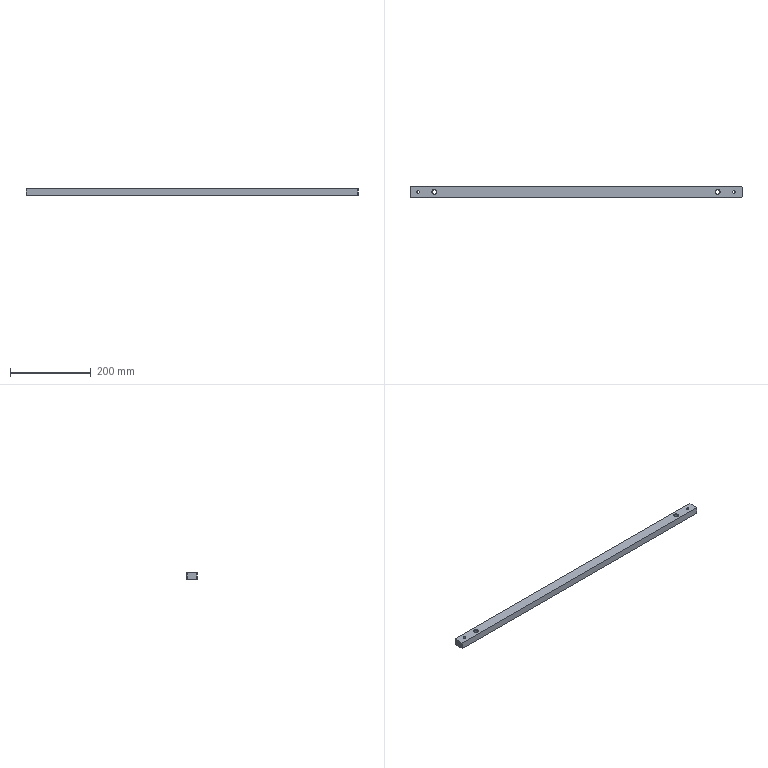Part | NX | features BREP 1 | 1 solid | 48 faces | box 820 x 26 x 17 mm | volume 357246 mm3 | cylinder 20 | cone 16 | plane 12 | commonest cylinder face diameters 3.3 x8 6.6 x4 10 x4 11 x4
STEP:
#1=CARTESIAN_POINT('',(395.5,0.,-1.5));
#2=VERTEX_POINT('',#1);
#3=CARTESIAN_POINT('',(384.5,0.,-1.5));
#4=VERTEX_POINT('',#3);
#5=CARTESIAN_POINT('',(390.,0.,-1.5));
#6=DIRECTION('',(0.,0.,-1.));
#7=DIRECTION('',(-1.,0.,0.));
#8=AXIS2_PLACEMENT_3D('',#5,#6,#7);
#9=CIRCLE('',#8,5.5);
#10=EDGE_CURVE('',#2,#4,#9,.T.);
#11=ORIENTED_EDGE('',*,*,#10,.F.);
#12=CARTESIAN_POINT('',(395.5,0.,-8.5));
#13=VERTEX_POINT('',#12);
#14=CARTESIAN_POINT('',(395.5,0.,-8.5));
#15=DIRECTION('',(0.,0.,-1.));
#16=VECTOR('',#15,1000.);
#17=LINE('',#14,#16);
#18=EDGE_CURVE('',#2,#13,#17,.T.);
#19=ORIENTED_EDGE('',*,*,#18,.T.);
#20=CARTESIAN_POINT('',(384.5,0.,-8.5));
#21=VERTEX_POINT('',#20);
#22=CARTESIAN_POINT('',(390.,0.,-8.5));
#23=DIRECTION('',(0.,0.,-1.));
#24=DIRECTION('',(-1.,0.,0.));
#25=AXIS2_PLACEMENT_3D('',#22,#23,#24);
#26=CIRCLE('',#25,5.5);
#27=EDGE_CURVE('',#13,#21,#26,.T.);
#28=ORIENTED_EDGE('',*,*,#27,.T.);
#29=CARTESIAN_POINT('',(384.5,0.,-8.5));
#30=DIRECTION('',(0.,0.,-1.));
#31=VECTOR('',#30,1000.);
#32=LINE('',#29,#31);
#33=EDGE_CURVE('',#4,#21,#32,.T.);
#34=ORIENTED_EDGE('',*,*,#33,.F.);
#35=EDGE_LOOP('',(#11,#19,#28,#34));
#36=FACE_BOUND('',#35,.T.);
#37=CARTESIAN_POINT('',(390.,0.,-8.5));
#38=DIRECTION('',(0.,0.,-1.));
#39=DIRECTION('',(-1.,0.,0.));
#40=AXIS2_PLACEMENT_3D('',#37,#38,#39);
#41=CYLINDRICAL_SURFACE('',#40,5.5);
#42=ADVANCED_FACE('',(#36),#41,.F.);
#43=CARTESIAN_POINT('',(393.3,0.,8.5));
#44=VERTEX_POINT('',#43);
#45=CARTESIAN_POINT('',(386.7,0.,8.5));
#46=VERTEX_POINT('',#45);
#47=CARTESIAN_POINT('',(390.,0.,8.5));
#48=DIRECTION('',(0.,0.,-1.));
#49=DIRECTION('',(-1.,0.,0.));
#50=AXIS2_PLACEMENT_3D('',#47,#48,#49);
#51=CIRCLE('',#50,3.3);
#52=EDGE_CURVE('',#44,#46,#51,.T.);
#53=ORIENTED_EDGE('',*,*,#52,.F.);
#54=CARTESIAN_POINT('',(393.3,0.,-1.5));
#55=VERTEX_POINT('',#54);
#56=CARTESIAN_POINT('',(393.3,0.,-8.5));
#57=DIRECTION('',(0.,0.,-1.));
#58=VECTOR('',#57,1000.);
#59=LINE('',#56,#58);
#60=EDGE_CURVE('',#44,#55,#59,.T.);
#61=ORIENTED_EDGE('',*,*,#60,.T.);
#62=CARTESIAN_POINT('',(386.7,0.,-1.5));
#63=VERTEX_POINT('',#62);
#64=CARTESIAN_POINT('',(390.,0.,-1.5));
#65=DIRECTION('',(0.,0.,-1.));
#66=DIRECTION('',(-1.,0.,0.));
#67=AXIS2_PLACEMENT_3D('',#64,#65,#66);
#68=CIRCLE('',#67,3.3);
#69=EDGE_CURVE('',#55,#63,#68,.T.);
#70=ORIENTED_EDGE('',*,*,#69,.T.);
#71=CARTESIAN_POINT('',(386.7,0.,-8.5));
#72=DIRECTION('',(0.,0.,-1.));
#73=VECTOR('',#72,1000.);
#74=LINE('',#71,#73);
#75=EDGE_CURVE('',#46,#63,#74,.T.);
#76=ORIENTED_EDGE('',*,*,#75,.F.);
#77=EDGE_LOOP('',(#53,#61,#70,#76));
#78=FACE_BOUND('',#77,.T.);
#79=CARTESIAN_POINT('',(390.,0.,-8.5));
#80=DIRECTION('',(0.,0.,-1.));
#81=DIRECTION('',(-1.,0.,0.));
#82=AXIS2_PLACEMENT_3D('',#79,#80,#81);
#83=CYLINDRICAL_SURFACE('',#82,3.3);
#84=ADVANCED_FACE('',(#78),#83,.F.);
#85=CARTESIAN_POINT('',(-386.7,0.,8.5));
#86=VERTEX_POINT('',#85);
#87=CARTESIAN_POINT('',(-393.3,0.,8.5));
#88=VERTEX_POINT('',#87);
#89=CARTESIAN_POINT('',(-390.,0.,8.5));
#90=DIRECTION('',(0.,0.,-1.));
#91=DIRECTION('',(-1.,0.,0.));
#92=AXIS2_PLACEMENT_3D('',#89,#90,#91);
#93=CIRCLE('',#92,3.3);
#94=EDGE_CURVE('',#86,#88,#93,.T.);
#95=ORIENTED_EDGE('',*,*,#94,.F.);
#96=CARTESIAN_POINT('',(-386.7,0.,-1.5));
#97=VERTEX_POINT('',#96);
#98=CARTESIAN_POINT('',(-386.7,0.,-8.5));
#99=DIRECTION('',(0.,0.,-1.));
#100=VECTOR('',#99,1000.);
#101=LINE('',#98,#100);
#102=EDGE_CURVE('',#86,#97,#101,.T.);
#103=ORIENTED_EDGE('',*,*,#102,.T.);
#104=CARTESIAN_POINT('',(-393.3,0.,-1.5));
#105=VERTEX_POINT('',#104);
#106=CARTESIAN_POINT('',(-390.,0.,-1.5));
#107=DIRECTION('',(0.,0.,-1.));
#108=DIRECTION('',(-1.,0.,0.));
#109=AXIS2_PLACEMENT_3D('',#106,#107,#108);
#110=CIRCLE('',#109,3.3);
#111=EDGE_CURVE('',#97,#105,#110,.T.);
#112=ORIENTED_EDGE('',*,*,#111,.T.);
#113=CARTESIAN_POINT('',(-393.3,0.,-8.5));
#114=DIRECTION('',(0.,0.,-1.));
#115=VECTOR('',#114,1000.);
#116=LINE('',#113,#115);
#117=EDGE_CURVE('',#88,#105,#116,.T.);
#118=ORIENTED_EDGE('',*,*,#117,.F.);
#119=EDGE_LOOP('',(#95,#103,#112,#118));
#120=FACE_BOUND('',#119,.T.);
#121=CARTESIAN_POINT('',(-390.,0.,-8.5));
#122=DIRECTION('',(0.,0.,-1.));
#123=DIRECTION('',(-1.,0.,0.));
#124=AXIS2_PLACEMENT_3D('',#121,#122,#123);
#125=CYLINDRICAL_SURFACE('',#124,3.3);
#126=ADVANCED_FACE('',(#120),#125,.F.);
#127=CARTESIAN_POINT('',(-384.5,0.,-1.5));
#128=VERTEX_POINT('',#127);
#129=CARTESIAN_POINT('',(-395.5,0.,-1.5));
#130=VERTEX_POINT('',#129);
#131=CARTESIAN_POINT('',(-390.,0.,-1.5));
#132=DIRECTION('',(0.,0.,-1.));
#133=DIRECTION('',(-1.,0.,0.));
#134=AXIS2_PLACEMENT_3D('',#131,#132,#133);
#135=CIRCLE('',#134,5.5);
#136=EDGE_CURVE('',#128,#130,#135,.T.);
#137=ORIENTED_EDGE('',*,*,#136,.F.);
#138=CARTESIAN_POINT('',(-384.5,0.,-8.5));
#139=VERTEX_POINT('',#138);
#140=CARTESIAN_POINT('',(-384.5,0.,-8.5));
#141=DIRECTION('',(0.,0.,-1.));
#142=VECTOR('',#141,1000.);
#143=LINE('',#140,#142);
#144=EDGE_CURVE('',#128,#139,#143,.T.);
#145=ORIENTED_EDGE('',*,*,#144,.T.);
#146=CARTESIAN_POINT('',(-395.5,0.,-8.5));
#147=VERTEX_POINT('',#146);
#148=CARTESIAN_POINT('',(-390.,0.,-8.5));
#149=DIRECTION('',(0.,0.,-1.));
#150=DIRECTION('',(-1.,0.,0.));
#151=AXIS2_PLACEMENT_3D('',#148,#149,#150);
#152=CIRCLE('',#151,5.5);
#153=EDGE_CURVE('',#139,#147,#152,.T.);
#154=ORIENTED_EDGE('',*,*,#153,.T.);
#155=CARTESIAN_POINT('',(-395.5,0.,-8.5));
#156=DIRECTION('',(0.,0.,-1.));
#157=VECTOR('',#156,1000.);
#158=LINE('',#155,#157);
#159=EDGE_CURVE('',#130,#147,#158,.T.);
#160=ORIENTED_EDGE('',*,*,#159,.F.);
#161=EDGE_LOOP('',(#137,#145,#154,#160));
#162=FACE_BOUND('',#161,.T.);
#163=CARTESIAN_POINT('',(-390.,0.,-8.5));
#164=DIRECTION('',(0.,0.,-1.));
#165=DIRECTION('',(-1.,0.,0.));
#166=AXIS2_PLACEMENT_3D('',#163,#164,#165);
#167=CYLINDRICAL_SURFACE('',#166,5.5);
#168=ADVANCED_FACE('',(#162),#167,.F.);
#169=CARTESIAN_POINT('',(-355.,0.,7.5));
#170=VERTEX_POINT('',#169);
#171=CARTESIAN_POINT('',(-345.,0.,7.5));
#172=VERTEX_POINT('',#171);
#173=CARTESIAN_POINT('',(-350.,0.,7.5));
#174=DIRECTION('',(0.,0.,1.));
#175=DIRECTION('',(-1.,0.,0.));
#176=AXIS2_PLACEMENT_3D('',#173,#174,#175);
#177=CIRCLE('',#176,5.);
#178=EDGE_CURVE('',#170,#172,#177,.T.);
#179=ORIENTED_EDGE('',*,*,#178,.F.);
#180=CARTESIAN_POINT('',(-356.,0.,8.5));
#181=VERTEX_POINT('',#180);
#182=CARTESIAN_POINT('',(-355.,0.,7.5));
#183=DIRECTION('',(-0.7071,0.,0.7071));
#184=VECTOR('',#183,1000.);
#185=LINE('',#182,#184);
#186=EDGE_CURVE('',#181,#170,#185,.F.);
#187=ORIENTED_EDGE('',*,*,#186,.F.);
#188=CARTESIAN_POINT('',(-344.,0.,8.5));
#189=VERTEX_POINT('',#188);
#190=CARTESIAN_POINT('',(-350.,0.,8.5));
#191=DIRECTION('',(0.,0.,-1.));
#192=DIRECTION('',(-1.,0.,0.));
#193=AXIS2_PLACEMENT_3D('',#190,#191,#192);
#194=CIRCLE('',#193,6.);
#195=EDGE_CURVE('',#189,#181,#194,.T.);
#196=ORIENTED_EDGE('',*,*,#195,.F.);
#197=CARTESIAN_POINT('',(-345.,0.,7.5));
#198=DIRECTION('',(0.7071,0.,0.7071));
#199=VECTOR('',#198,1000.);
#200=LINE('',#197,#199);
#201=EDGE_CURVE('',#189,#172,#200,.F.);
#202=ORIENTED_EDGE('',*,*,#201,.T.);
#203=EDGE_LOOP('',(#179,#187,#196,#202));
#204=FACE_BOUND('',#203,.T.);
#205=CARTESIAN_POINT('',(-350.,0.,7.5));
#206=DIRECTION('',(0.,0.,1.));
#207=DIRECTION('',(1.,0.,0.));
#208=AXIS2_PLACEMENT_3D('',#205,#206,#207);
#209=CONICAL_SURFACE('',#208,5.,0.7854);
#210=ADVANCED_FACE('',(#204),#209,.F.);
#211=CARTESIAN_POINT('',(-345.,0.,-7.5));
#212=VERTEX_POINT('',#211);
#213=CARTESIAN_POINT('',(-355.,0.,-7.5));
#214=VERTEX_POINT('',#213);
#215=CARTESIAN_POINT('',(-350.,0.,-7.5));
#216=DIRECTION('',(0.,0.,-1.));
#217=DIRECTION('',(-1.,0.,0.));
#218=AXIS2_PLACEMENT_3D('',#215,#216,#217);
#219=CIRCLE('',#218,5.);
#220=EDGE_CURVE('',#212,#214,#219,.T.);
#221=ORIENTED_EDGE('',*,*,#220,.F.);
#222=CARTESIAN_POINT('',(-344.,0.,-8.5));
#223=VERTEX_POINT('',#222);
#224=CARTESIAN_POINT('',(-345.,0.,-7.5));
#225=DIRECTION('',(0.7071,0.,-0.7071));
#226=VECTOR('',#225,1000.);
#227=LINE('',#224,#226);
#228=EDGE_CURVE('',#212,#223,#227,.T.);
#229=ORIENTED_EDGE('',*,*,#228,.T.);
#230=CARTESIAN_POINT('',(-356.,0.,-8.5));
#231=VERTEX_POINT('',#230);
#232=CARTESIAN_POINT('',(-350.,0.,-8.5));
#233=DIRECTION('',(0.,0.,1.));
#234=DIRECTION('',(-1.,0.,0.));
#235=AXIS2_PLACEMENT_3D('',#232,#233,#234);
#236=CIRCLE('',#235,6.);
#237=EDGE_CURVE('',#231,#223,#236,.T.);
#238=ORIENTED_EDGE('',*,*,#237,.F.);
#239=CARTESIAN_POINT('',(-355.,0.,-7.5));
#240=DIRECTION('',(-0.7071,0.,-0.7071));
#241=VECTOR('',#240,1000.);
#242=LINE('',#239,#241);
#243=EDGE_CURVE('',#214,#231,#242,.T.);
#244=ORIENTED_EDGE('',*,*,#243,.F.);
#245=EDGE_LOOP('',(#221,#229,#238,#244));
#246=FACE_BOUND('',#245,.T.);
#247=CARTESIAN_POINT('',(-350.,0.,-7.5));
#248=DIRECTION('',(0.,0.,-1.));
#249=DIRECTION('',(-1.,0.,0.));
#250=AXIS2_PLACEMENT_3D('',#247,#248,#249);
#251=CONICAL_SURFACE('',#250,5.,0.7854);
#252=ADVANCED_FACE('',(#246),#251,.F.);
#253=CARTESIAN_POINT('',(345.,0.,7.5));
#254=VERTEX_POINT('',#253);
#255=CARTESIAN_POINT('',(355.,0.,7.5));
#256=VERTEX_POINT('',#255);
#257=CARTESIAN_POINT('',(350.,0.,7.5));
#258=DIRECTION('',(0.,0.,1.));
#259=DIRECTION('',(-1.,0.,0.));
#260=AXIS2_PLACEMENT_3D('',#257,#258,#259);
#261=CIRCLE('',#260,5.);
#262=EDGE_CURVE('',#254,#256,#261,.T.);
#263=ORIENTED_EDGE('',*,*,#262,.F.);
#264=CARTESIAN_POINT('',(344.,0.,8.5));
#265=VERTEX_POINT('',#264);
#266=CARTESIAN_POINT('',(345.,0.,7.5));
#267=DIRECTION('',(-0.7071,0.,0.7071));
#268=VECTOR('',#267,1000.);
#269=LINE('',#266,#268);
#270=EDGE_CURVE('',#265,#254,#269,.F.);
#271=ORIENTED_EDGE('',*,*,#270,.F.);
#272=CARTESIAN_POINT('',(356.,0.,8.5));
#273=VERTEX_POINT('',#272);
#274=CARTESIAN_POINT('',(350.,0.,8.5));
#275=DIRECTION('',(0.,0.,-1.));
#276=DIRECTION('',(-1.,0.,0.));
#277=AXIS2_PLACEMENT_3D('',#274,#275,#276);
#278=CIRCLE('',#277,6.);
#279=EDGE_CURVE('',#273,#265,#278,.T.);
#280=ORIENTED_EDGE('',*,*,#279,.F.);
#281=CARTESIAN_POINT('',(355.,0.,7.5));
#282=DIRECTION('',(0.7071,0.,0.7071));
#283=VECTOR('',#282,1000.);
#284=LINE('',#281,#283);
#285=EDGE_CURVE('',#273,#256,#284,.F.);
#286=ORIENTED_EDGE('',*,*,#285,.T.);
#287=EDGE_LOOP('',(#263,#271,#280,#286));
#288=FACE_BOUND('',#287,.T.);
#289=CARTESIAN_POINT('',(350.,0.,7.5));
#290=DIRECTION('',(0.,0.,1.));
#291=DIRECTION('',(1.,0.,0.));
#292=AXIS2_PLACEMENT_3D('',#289,#290,#291);
#293=CONICAL_SURFACE('',#292,5.,0.7854);
#294=ADVANCED_FACE('',(#288),#293,.F.);
#295=CARTESIAN_POINT('',(355.,0.,-7.5));
#296=VERTEX_POINT('',#295);
#297=CARTESIAN_POINT('',(345.,0.,-7.5));
#298=VERTEX_POINT('',#297);
#299=CARTESIAN_POINT('',(350.,0.,-7.5));
#300=DIRECTION('',(0.,0.,-1.));
#301=DIRECTION('',(-1.,0.,0.));
#302=AXIS2_PLACEMENT_3D('',#299,#300,#301);
#303=CIRCLE('',#302,5.);
#304=EDGE_CURVE('',#296,#298,#303,.T.);
#305=ORIENTED_EDGE('',*,*,#304,.F.);
#306=CARTESIAN_POINT('',(356.,0.,-8.5));
#307=VERTEX_POINT('',#306);
#308=CARTESIAN_POINT('',(355.,0.,-7.5));
#309=DIRECTION('',(0.7071,0.,-0.7071));
#310=VECTOR('',#309,1000.);
#311=LINE('',#308,#310);
#312=EDGE_CURVE('',#296,#307,#311,.T.);
#313=ORIENTED_EDGE('',*,*,#312,.T.);
#314=CARTESIAN_POINT('',(344.,0.,-8.5));
#315=VERTEX_POINT('',#314);
#316=CARTESIAN_POINT('',(350.,0.,-8.5));
#317=DIRECTION('',(0.,0.,1.));
#318=DIRECTION('',(-1.,0.,0.));
#319=AXIS2_PLACEMENT_3D('',#316,#317,#318);
#320=CIRCLE('',#319,6.);
#321=EDGE_CURVE('',#315,#307,#320,.T.);
#322=ORIENTED_EDGE('',*,*,#321,.F.);
#323=CARTESIAN_POINT('',(345.,0.,-7.5));
#324=DIRECTION('',(-0.7071,0.,-0.7071));
#325=VECTOR('',#324,1000.);
#326=LINE('',#323,#325);
#327=EDGE_CURVE('',#298,#315,#326,.T.);
#328=ORIENTED_EDGE('',*,*,#327,.F.);
#329=EDGE_LOOP('',(#305,#313,#322,#328));
#330=FACE_BOUND('',#329,.T.);
#331=CARTESIAN_POINT('',(350.,0.,-7.5));
#332=DIRECTION('',(0.,0.,-1.));
#333=DIRECTION('',(-1.,0.,0.));
#334=AXIS2_PLACEMENT_3D('',#331,#332,#333);
#335=CONICAL_SURFACE('',#334,5.,0.7854);
#336=ADVANCED_FACE('',(#330),#335,.F.);
#337=ORIENTED_EDGE('',*,*,#304,.T.);
#338=CARTESIAN_POINT('',(345.,0.,-174.5));
#339=DIRECTION('',(0.,0.,1.));
#340=VECTOR('',#339,1000.);
#341=LINE('',#338,#340);
#342=EDGE_CURVE('',#254,#298,#341,.F.);
#343=ORIENTED_EDGE('',*,*,#342,.F.);
#344=ORIENTED_EDGE('',*,*,#262,.T.);
#345=CARTESIAN_POINT('',(355.,0.,-174.5));
#346=DIRECTION('',(0.,0.,1.));
#347=VECTOR('',#346,1000.);
#348=LINE('',#345,#347);
#349=EDGE_CURVE('',#256,#296,#348,.F.);
#350=ORIENTED_EDGE('',*,*,#349,.T.);
#351=EDGE_LOOP('',(#337,#343,#344,#350));
#352=FACE_BOUND('',#351,.T.);
#353=CARTESIAN_POINT('',(350.,0.,-174.5));
#354=DIRECTION('',(0.,0.,1.));
#355=DIRECTION('',(1.,0.,0.));
#356=AXIS2_PLACEMENT_3D('',#353,#354,#355);
#357=CYLINDRICAL_SURFACE('',#356,5.);
#358=ADVANCED_FACE('',(#352),#357,.F.);
#359=ORIENTED_EDGE('',*,*,#220,.T.);
#360=CARTESIAN_POINT('',(-355.,0.,-174.5));
#361=DIRECTION('',(0.,0.,1.));
#362=VECTOR('',#361,1000.);
#363=LINE('',#360,#362);
#364=EDGE_CURVE('',#170,#214,#363,.F.);
#365=ORIENTED_EDGE('',*,*,#364,.F.);
#366=ORIENTED_EDGE('',*,*,#178,.T.);
#367=CARTESIAN_POINT('',(-345.,0.,-174.5));
#368=DIRECTION('',(0.,0.,1.));
#369=VECTOR('',#368,1000.);
#370=LINE('',#367,#369);
#371=EDGE_CURVE('',#172,#212,#370,.F.);
#372=ORIENTED_EDGE('',*,*,#371,.T.);
#373=EDGE_LOOP('',(#359,#365,#366,#372));
#374=FACE_BOUND('',#373,.T.);
#375=CARTESIAN_POINT('',(-350.,0.,-174.5));
#376=DIRECTION('',(0.,0.,1.));
#377=DIRECTION('',(1.,0.,0.));
#378=AXIS2_PLACEMENT_3D('',#375,#376,#377);
#379=CYLINDRICAL_SURFACE('',#378,5.);
#380=ADVANCED_FACE('',(#374),#379,.F.);
#381=CARTESIAN_POINT('',(-395.292,1.5,-1.624));
#382=VERTEX_POINT('',#381);
#383=CARTESIAN_POINT('',(-395.,2.291,-1.65));
#384=VERTEX_POINT('',#383);
#385=CARTESIAN_POINT('',(-395.292,1.5,-1.624));
#386=CARTESIAN_POINT('',(-395.214,1.772,-1.638));
#387=CARTESIAN_POINT('',(-395.117,2.036,-1.65));
#388=CARTESIAN_POINT('',(-395.,2.291,-1.65));
#389=B_SPLINE_CURVE_WITH_KNOTS('',3,(#385,#386,#387,#388),.UNSPECIFIED.,.F.,.F.,(4,4),(0.,1.),.UNSPECIFIED.);
#390=EDGE_CURVE('',#382,#384,#389,.T.);
#391=ORIENTED_EDGE('',*,*,#390,.T.);
#392=CARTESIAN_POINT('',(-395.,13.,-1.65));
#393=VERTEX_POINT('',#392);
#394=CARTESIAN_POINT('',(-395.,13.,-1.65));
#395=DIRECTION('',(0.,1.,0.));
#396=VECTOR('',#395,1000.);
#397=LINE('',#394,#396);
#398=EDGE_CURVE('',#384,#393,#397,.T.);
#399=ORIENTED_EDGE('',*,*,#398,.T.);
#400=CARTESIAN_POINT('',(-395.,13.,1.65));
#401=VERTEX_POINT('',#400);
#402=CARTESIAN_POINT('',(-395.,13.,0.));
#403=DIRECTION('',(0.,1.,0.));
#404=DIRECTION('',(0.,0.,1.));
#405=AXIS2_PLACEMENT_3D('',#402,#403,#404);
#406=CIRCLE('',#405,1.65);
#407=EDGE_CURVE('',#393,#401,#406,.T.);
#408=ORIENTED_EDGE('',*,*,#407,.T.);
#409=CARTESIAN_POINT('',(-395.,1.5,1.65));
#410=VERTEX_POINT('',#409);
#411=CARTESIAN_POINT('',(-395.,13.,1.65));
#412=DIRECTION('',(0.,1.,0.));
#413=VECTOR('',#412,1000.);
#414=LINE('',#411,#413);
#415=EDGE_CURVE('',#410,#401,#414,.T.);
#416=ORIENTED_EDGE('',*,*,#415,.F.);
#417=CARTESIAN_POINT('',(-395.,1.5,0.));
#418=DIRECTION('',(0.,1.,0.));
#419=DIRECTION('',(0.,0.,1.));
#420=AXIS2_PLACEMENT_3D('',#417,#418,#419);
#421=CIRCLE('',#420,1.65);
#422=EDGE_CURVE('',#382,#410,#421,.T.);
#423=ORIENTED_EDGE('',*,*,#422,.F.);
#424=EDGE_LOOP('',(#391,#399,#408,#416,#423));
#425=FACE_BOUND('',#424,.T.);
#426=CARTESIAN_POINT('',(-395.,13.,0.));
#427=DIRECTION('',(0.,1.,0.));
#428=DIRECTION('',(0.,0.,1.));
#429=AXIS2_PLACEMENT_3D('',#426,#427,#428);
#430=CYLINDRICAL_SURFACE('',#429,1.65);
#431=ADVANCED_FACE('',(#425),#430,.F.);
#432=CARTESIAN_POINT('',(-395.,0.5086,0.));
#433=VERTEX_POINT('',#432);
#434=CARTESIAN_POINT('',(-395.,1.5,1.65));
#435=DIRECTION('',(0.,0.515,0.8572));
#436=VECTOR('',#435,1000.);
#437=LINE('',#434,#436);
#438=EDGE_CURVE('',#410,#433,#437,.F.);
#439=ORIENTED_EDGE('',*,*,#438,.T.);
#440=CARTESIAN_POINT('',(-395.,1.41,-1.5));
#441=VERTEX_POINT('',#440);
#442=CARTESIAN_POINT('',(-395.,1.5,-1.65));
#443=DIRECTION('',(0.,0.515,-0.8572));
#444=VECTOR('',#443,1000.);
#445=LINE('',#442,#444);
#446=EDGE_CURVE('',#441,#433,#445,.F.);
#447=ORIENTED_EDGE('',*,*,#446,.F.);
#448=CARTESIAN_POINT('',(-395.311,1.429,-1.5));
#449=VERTEX_POINT('',#448);
#450=CARTESIAN_POINT('',(-395.311,1.429,-1.5));
#451=CARTESIAN_POINT('',(-395.206,1.416,-1.5));
#452=CARTESIAN_POINT('',(-395.103,1.41,-1.5));
#453=CARTESIAN_POINT('',(-395.,1.41,-1.5));
#454=B_SPLINE_CURVE_WITH_KNOTS('',3,(#450,#451,#452,#453),.UNSPECIFIED.,.F.,.F.,(4,4),(0.,1.),.UNSPECIFIED.);
#455=EDGE_CURVE('',#441,#449,#454,.F.);
#456=ORIENTED_EDGE('',*,*,#455,.T.);
#457=CARTESIAN_POINT('',(-395.311,1.429,-1.5));
#458=CARTESIAN_POINT('',(-395.305,1.453,-1.541));
#459=CARTESIAN_POINT('',(-395.298,1.476,-1.583));
#460=CARTESIAN_POINT('',(-395.292,1.5,-1.624));
#461=B_SPLINE_CURVE_WITH_KNOTS('',3,(#457,#458,#459,#460),.UNSPECIFIED.,.F.,.F.,(4,4),(0.00001764,0.0001619),.UNSPECIFIED.);
#462=EDGE_CURVE('',#449,#382,#461,.T.);
#463=ORIENTED_EDGE('',*,*,#462,.T.);
#464=ORIENTED_EDGE('',*,*,#422,.T.);
#465=EDGE_LOOP('',(#439,#447,#456,#463,#464));
#466=FACE_BOUND('',#465,.T.);
#467=CARTESIAN_POINT('',(-395.,1.5,0.));
#468=DIRECTION('',(0.,1.,0.));
#469=DIRECTION('',(0.,0.,1.));
#470=AXIS2_PLACEMENT_3D('',#467,#468,#469);
#471=CONICAL_SURFACE('',#470,1.65,1.03);
#472=ADVANCED_FACE('',(#466),#471,.F.);
#473=CARTESIAN_POINT('',(-131.,1.5,-1.65));
#474=VERTEX_POINT('',#473);
#475=CARTESIAN_POINT('',(-131.,1.5,1.65));
#476=VERTEX_POINT('',#475);
#477=CARTESIAN_POINT('',(-131.,1.5,0.));
#478=DIRECTION('',(0.,1.,0.));
#479=DIRECTION('',(0.,0.,1.));
#480=AXIS2_PLACEMENT_3D('',#477,#478,#479);
#481=CIRCLE('',#480,1.65);
#482=EDGE_CURVE('',#474,#476,#481,.T.);
#483=ORIENTED_EDGE('',*,*,#482,.F.);
#484=CARTESIAN_POINT('',(-131.,13.,-1.65));
#485=VERTEX_POINT('',#484);
#486=CARTESIAN_POINT('',(-131.,13.,-1.65));
#487=DIRECTION('',(0.,1.,0.));
#488=VECTOR('',#487,1000.);
#489=LINE('',#486,#488);
#490=EDGE_CURVE('',#485,#474,#489,.F.);
#491=ORIENTED_EDGE('',*,*,#490,.F.);
#492=CARTESIAN_POINT('',(-131.,13.,1.65));
#493=VERTEX_POINT('',#492);
#494=CARTESIAN_POINT('',(-131.,13.,0.));
#495=DIRECTION('',(0.,1.,0.));
#496=DIRECTION('',(0.,0.,1.));
#497=AXIS2_PLACEMENT_3D('',#494,#495,#496);
#498=CIRCLE('',#497,1.65);
#499=EDGE_CURVE('',#485,#493,#498,.T.);
#500=ORIENTED_EDGE('',*,*,#499,.T.);
#501=CARTESIAN_POINT('',(-131.,13.,1.65));
#502=DIRECTION('',(0.,1.,0.));
#503=VECTOR('',#502,1000.);
#504=LINE('',#501,#503);
#505=EDGE_CURVE('',#493,#476,#504,.F.);
#506=ORIENTED_EDGE('',*,*,#505,.T.);
#507=EDGE_LOOP('',(#483,#491,#500,#506));
#508=FACE_BOUND('',#507,.T.);
#509=CARTESIAN_POINT('',(-131.,13.,0.));
#510=DIRECTION('',(0.,1.,0.));
#511=DIRECTION('',(0.,0.,1.));
#512=AXIS2_PLACEMENT_3D('',#509,#510,#511);
#513=CYLINDRICAL_SURFACE('',#512,1.65);
#514=ADVANCED_FACE('',(#508),#513,.F.);
#515=CARTESIAN_POINT('',(-131.,0.5086,0.));
#516=VERTEX_POINT('',#515);
#517=CARTESIAN_POINT('',(-131.,1.5,1.65));
#518=DIRECTION('',(0.,0.515,0.8572));
#519=VECTOR('',#518,1000.);
#520=LINE('',#517,#519);
#521=EDGE_CURVE('',#476,#516,#520,.F.);
#522=ORIENTED_EDGE('',*,*,#521,.T.);
#523=CARTESIAN_POINT('',(-131.,1.5,-1.65));
#524=DIRECTION('',(0.,0.515,-0.8572));
#525=VECTOR('',#524,1000.);
#526=LINE('',#523,#525);
#527=EDGE_CURVE('',#474,#516,#526,.F.);
#528=ORIENTED_EDGE('',*,*,#527,.F.);
#529=ORIENTED_EDGE('',*,*,#482,.T.);
#530=EDGE_LOOP('',(#522,#528,#529));
#531=FACE_BOUND('',#530,.T.);
#532=CARTESIAN_POINT('',(-131.,1.5,0.));
#533=DIRECTION('',(0.,1.,0.));
#534=DIRECTION('',(0.,0.,1.));
#535=AXIS2_PLACEMENT_3D('',#532,#533,#534);
#536=CONICAL_SURFACE('',#535,1.65,1.03);
#537=ADVANCED_FACE('',(#531),#536,.F.);
#538=CARTESIAN_POINT('',(133.,1.5,-1.65));
#539=VERTEX_POINT('',#538);
#540=CARTESIAN_POINT('',(133.,1.5,1.65));
#541=VERTEX_POINT('',#540);
#542=CARTESIAN_POINT('',(133.,1.5,0.));
#543=DIRECTION('',(0.,1.,0.));
#544=DIRECTION('',(0.,0.,1.));
#545=AXIS2_PLACEMENT_3D('',#542,#543,#544);
#546=CIRCLE('',#545,1.65);
#547=EDGE_CURVE('',#539,#541,#546,.T.);
#548=ORIENTED_EDGE('',*,*,#547,.F.);
#549=CARTESIAN_POINT('',(133.,13.,-1.65));
#550=VERTEX_POINT('',#549);
#551=CARTESIAN_POINT('',(133.,13.,-1.65));
#552=DIRECTION('',(0.,1.,0.));
#553=VECTOR('',#552,1000.);
#554=LINE('',#551,#553);
#555=EDGE_CURVE('',#550,#539,#554,.F.);
#556=ORIENTED_EDGE('',*,*,#555,.F.);
#557=CARTESIAN_POINT('',(133.,13.,1.65));
#558=VERTEX_POINT('',#557);
#559=CARTESIAN_POINT('',(133.,13.,0.));
#560=DIRECTION('',(0.,1.,0.));
#561=DIRECTION('',(0.,0.,1.));
#562=AXIS2_PLACEMENT_3D('',#559,#560,#561);
#563=CIRCLE('',#562,1.65);
#564=EDGE_CURVE('',#550,#558,#563,.T.);
#565=ORIENTED_EDGE('',*,*,#564,.T.);
#566=CARTESIAN_POINT('',(133.,13.,1.65));
#567=DIRECTION('',(0.,1.,0.));
#568=VECTOR('',#567,1000.);
#569=LINE('',#566,#568);
#570=EDGE_CURVE('',#558,#541,#569,.F.);
#571=ORIENTED_EDGE('',*,*,#570,.T.);
#572=EDGE_LOOP('',(#548,#556,#565,#571));
#573=FACE_BOUND('',#572,.T.);
#574=CARTESIAN_POINT('',(133.,13.,0.));
#575=DIRECTION('',(0.,1.,0.));
#576=DIRECTION('',(0.,0.,1.));
#577=AXIS2_PLACEMENT_3D('',#574,#575,#576);
#578=CYLINDRICAL_SURFACE('',#577,1.65);
#579=ADVANCED_FACE('',(#573),#578,.F.);
#580=CARTESIAN_POINT('',(133.,0.5086,0.));
#581=VERTEX_POINT('',#580);
#582=CARTESIAN_POINT('',(133.,1.5,1.65));
#583=DIRECTION('',(0.,0.515,0.8572));
#584=VECTOR('',#583,1000.);
#585=LINE('',#582,#584);
#586=EDGE_CURVE('',#541,#581,#585,.F.);
#587=ORIENTED_EDGE('',*,*,#586,.T.);
#588=CARTESIAN_POINT('',(133.,1.5,-1.65));
#589=DIRECTION('',(0.,0.515,-0.8572));
#590=VECTOR('',#589,1000.);
#591=LINE('',#588,#590);
#592=EDGE_CURVE('',#539,#581,#591,.F.);
#593=ORIENTED_EDGE('',*,*,#592,.F.);
#594=ORIENTED_EDGE('',*,*,#547,.T.);
#595=EDGE_LOOP('',(#587,#593,#594));
#596=FACE_BOUND('',#595,.T.);
#597=CARTESIAN_POINT('',(133.,1.5,0.));
#598=DIRECTION('',(0.,1.,0.));
#599=DIRECTION('',(0.,0.,1.));
#600=AXIS2_PLACEMENT_3D('',#597,#598,#599);
#601=CONICAL_SURFACE('',#600,1.65,1.03);
#602=ADVANCED_FACE('',(#596),#601,.F.);
#603=CARTESIAN_POINT('',(397.,1.5,-1.65));
#604=VERTEX_POINT('',#603);
#605=CARTESIAN_POINT('',(397.,1.5,1.65));
#606=VERTEX_POINT('',#605);
#607=CARTESIAN_POINT('',(397.,1.5,0.));
#608=DIRECTION('',(0.,1.,0.));
#609=DIRECTION('',(0.,0.,1.));
#610=AXIS2_PLACEMENT_3D('',#607,#608,#609);
#611=CIRCLE('',#610,1.65);
#612=EDGE_CURVE('',#604,#606,#611,.T.);
#613=ORIENTED_EDGE('',*,*,#612,.F.);
#614=CARTESIAN_POINT('',(397.,13.,-1.65));
#615=VERTEX_POINT('',#614);
#616=CARTESIAN_POINT('',(397.,13.,-1.65));
#617=DIRECTION('',(0.,1.,0.));
#618=VECTOR('',#617,1000.);
#619=LINE('',#616,#618);
#620=EDGE_CURVE('',#615,#604,#619,.F.);
#621=ORIENTED_EDGE('',*,*,#620,.F.);
#622=CARTESIAN_POINT('',(397.,13.,1.65));
#623=VERTEX_POINT('',#622);
#624=CARTESIAN_POINT('',(397.,13.,0.));
#625=DIRECTION('',(0.,1.,0.));
#626=DIRECTION('',(0.,0.,1.));
#627=AXIS2_PLACEMENT_3D('',#624,#625,#626);
#628=CIRCLE('',#627,1.65);
#629=EDGE_CURVE('',#615,#623,#628,.T.);
#630=ORIENTED_EDGE('',*,*,#629,.T.);
#631=CARTESIAN_POINT('',(397.,13.,1.65));
#632=DIRECTION('',(0.,1.,0.));
#633=VECTOR('',#632,1000.);
#634=LINE('',#631,#633);
#635=EDGE_CURVE('',#623,#606,#634,.F.);
#636=ORIENTED_EDGE('',*,*,#635,.T.);
#637=EDGE_LOOP('',(#613,#621,#630,#636));
#638=FACE_BOUND('',#637,.T.);
#639=CARTESIAN_POINT('',(397.,13.,0.));
#640=DIRECTION('',(0.,1.,0.));
#641=DIRECTION('',(0.,0.,1.));
#642=AXIS2_PLACEMENT_3D('',#639,#640,#641);
#643=CYLINDRICAL_SURFACE('',#642,1.65);
#644=ADVANCED_FACE('',(#638),#643,.F.);
#645=CARTESIAN_POINT('',(397.,0.5086,0.));
#646=VERTEX_POINT('',#645);
#647=CARTESIAN_POINT('',(397.,1.5,1.65));
#648=DIRECTION('',(0.,0.515,0.8572));
#649=VECTOR('',#648,1000.);
#650=LINE('',#647,#649);
#651=EDGE_CURVE('',#606,#646,#650,.F.);
#652=ORIENTED_EDGE('',*,*,#651,.T.);
#653=CARTESIAN_POINT('',(397.,1.5,-1.65));
#654=DIRECTION('',(0.,0.515,-0.8572));
#655=VECTOR('',#654,1000.);
#656=LINE('',#653,#655);
#657=EDGE_CURVE('',#604,#646,#656,.F.);
#658=ORIENTED_EDGE('',*,*,#657,.F.);
#659=ORIENTED_EDGE('',*,*,#612,.T.);
#660=EDGE_LOOP('',(#652,#658,#659));
#661=FACE_BOUND('',#660,.T.);
#662=CARTESIAN_POINT('',(397.,1.5,0.));
#663=DIRECTION('',(0.,1.,0.));
#664=DIRECTION('',(0.,0.,1.));
#665=AXIS2_PLACEMENT_3D('',#662,#663,#664);
#666=CONICAL_SURFACE('',#665,1.65,1.03);
#667=ADVANCED_FACE('',(#661),#666,.F.);
#668=CARTESIAN_POINT('',(410.,-12.,8.5));
#669=VERTEX_POINT('',#668);
#670=CARTESIAN_POINT('',(410.,12.,8.5));
#671=VERTEX_POINT('',#670);
#672=CARTESIAN_POINT('',(410.,-13.,8.5));
#673=DIRECTION('',(0.,1.,0.));
#674=VECTOR('',#673,1000.);
#675=LINE('',#672,#674);
#676=EDGE_CURVE('',#669,#671,#675,.T.);
#677=ORIENTED_EDGE('',*,*,#676,.F.);
#678=CARTESIAN_POINT('',(410.,-12.,-8.5));
#679=VERTEX_POINT('',#678);
#680=CARTESIAN_POINT('',(410.,-12.,8.5));
#681=DIRECTION('',(0.,0.,-1.));
#682=VECTOR('',#681,1000.);
#683=LINE('',#680,#682);
#684=EDGE_CURVE('',#669,#679,#683,.T.);
#685=ORIENTED_EDGE('',*,*,#684,.T.);
#686=CARTESIAN_POINT('',(410.,12.,-8.5));
#687=VERTEX_POINT('',#686);
#688=CARTESIAN_POINT('',(410.,-13.,-8.5));
#689=DIRECTION('',(0.,1.,0.));
#690=VECTOR('',#689,1000.);
#691=LINE('',#688,#690);
#692=EDGE_CURVE('',#679,#687,#691,.T.);
#693=ORIENTED_EDGE('',*,*,#692,.T.);
#694=CARTESIAN_POINT('',(410.,12.,8.5));
#695=DIRECTION('',(0.,0.,1.));
#696=VECTOR('',#695,1000.);
#697=LINE('',#694,#696);
#698=EDGE_CURVE('',#687,#671,#697,.T.);
#699=ORIENTED_EDGE('',*,*,#698,.T.);
#700=EDGE_LOOP('',(#677,#685,#693,#699));
#701=FACE_BOUND('',#700,.T.);
#702=CARTESIAN_POINT('',(410.,-13.,8.5));
#703=DIRECTION('',(-1.,0.,0.));
#704=DIRECTION('',(0.,0.,1.));
#705=AXIS2_PLACEMENT_3D('',#702,#703,#704);
#706=PLANE('',#705);
#707=ADVANCED_FACE('',(#701),#706,.F.);
#708=CARTESIAN_POINT('',(409.,13.,8.5));
#709=VERTEX_POINT('',#708);
#710=CARTESIAN_POINT('',(-409.,13.,8.5));
#711=VERTEX_POINT('',#710);
#712=CARTESIAN_POINT('',(-410.,13.,8.5));
#713=DIRECTION('',(-1.,0.,0.));
#714=VECTOR('',#713,1000.);
#715=LINE('',#712,#714);
#716=EDGE_CURVE('',#709,#711,#715,.T.);
#717=ORIENTED_EDGE('',*,*,#716,.F.);
#718=CARTESIAN_POINT('',(409.,13.,-8.5));
#719=VERTEX_POINT('',#718);
#720=CARTESIAN_POINT('',(409.,13.,8.5));
#721=DIRECTION('',(0.,0.,-1.));
#722=VECTOR('',#721,1000.);
#723=LINE('',#720,#722);
#724=EDGE_CURVE('',#709,#719,#723,.T.);
#725=ORIENTED_EDGE('',*,*,#724,.T.);
#726=CARTESIAN_POINT('',(-409.,13.,-8.5));
#727=VERTEX_POINT('',#726);
#728=CARTESIAN_POINT('',(-410.,13.,-8.5));
#729=DIRECTION('',(-1.,0.,0.));
#730=VECTOR('',#729,1000.);
#731=LINE('',#728,#730);
#732=EDGE_CURVE('',#719,#727,#731,.T.);
#733=ORIENTED_EDGE('',*,*,#732,.T.);
#734=CARTESIAN_POINT('',(-409.,13.,8.5));
#735=DIRECTION('',(0.,0.,1.));
#736=VECTOR('',#735,1000.);
#737=LINE('',#734,#736);
#738=EDGE_CURVE('',#727,#711,#737,.T.);
#739=ORIENTED_EDGE('',*,*,#738,.T.);
#740=EDGE_LOOP('',(#717,#725,#733,#739));
#741=FACE_BOUND('',#740,.T.);
#742=CARTESIAN_POINT('',(-395.,13.,0.));
#743=DIRECTION('',(0.,1.,0.));
#744=DIRECTION('',(0.,0.,1.));
#745=AXIS2_PLACEMENT_3D('',#742,#743,#744);
#746=CIRCLE('',#745,1.65);
#747=EDGE_CURVE('',#401,#393,#746,.T.);
#748=ORIENTED_EDGE('',*,*,#747,.F.);
#749=ORIENTED_EDGE('',*,*,#407,.F.);
#750=EDGE_LOOP('',(#748,#749));
#751=FACE_BOUND('',#750,.T.);
#752=CARTESIAN_POINT('',(-131.,13.,0.));
#753=DIRECTION('',(0.,1.,0.));
#754=DIRECTION('',(0.,0.,1.));
#755=AXIS2_PLACEMENT_3D('',#752,#753,#754);
#756=CIRCLE('',#755,1.65);
#757=EDGE_CURVE('',#493,#485,#756,.T.);
#758=ORIENTED_EDGE('',*,*,#757,.F.);
#759=ORIENTED_EDGE('',*,*,#499,.F.);
#760=EDGE_LOOP('',(#758,#759));
#761=FACE_BOUND('',#760,.T.);
#762=CARTESIAN_POINT('',(133.,13.,0.));
#763=DIRECTION('',(0.,1.,0.));
#764=DIRECTION('',(0.,0.,1.));
#765=AXIS2_PLACEMENT_3D('',#762,#763,#764);
#766=CIRCLE('',#765,1.65);
#767=EDGE_CURVE('',#558,#550,#766,.T.);
#768=ORIENTED_EDGE('',*,*,#767,.F.);
#769=ORIENTED_EDGE('',*,*,#564,.F.);
#770=EDGE_LOOP('',(#768,#769));
#771=FACE_BOUND('',#770,.T.);
#772=CARTESIAN_POINT('',(397.,13.,0.));
#773=DIRECTION('',(0.,1.,0.));
#774=DIRECTION('',(0.,0.,1.));
#775=AXIS2_PLACEMENT_3D('',#772,#773,#774);
#776=CIRCLE('',#775,1.65);
#777=EDGE_CURVE('',#623,#615,#776,.T.);
#778=ORIENTED_EDGE('',*,*,#777,.F.);
#779=ORIENTED_EDGE('',*,*,#629,.F.);
#780=EDGE_LOOP('',(#778,#779));
#781=FACE_BOUND('',#780,.T.);
#782=CARTESIAN_POINT('',(-410.,13.,8.5));
#783=DIRECTION('',(0.,-1.,0.));
#784=DIRECTION('',(0.,0.,-1.));
#785=AXIS2_PLACEMENT_3D('',#782,#783,#784);
#786=PLANE('',#785);
#787=ADVANCED_FACE('',(#741,#751,#761,#771,#781),#786,.F.);
#788=CARTESIAN_POINT('',(-410.,12.,-8.5));
#789=VERTEX_POINT('',#788);
#790=CARTESIAN_POINT('',(-410.,-12.,-8.5));
#791=VERTEX_POINT('',#790);
#792=CARTESIAN_POINT('',(-410.,-13.,-8.5));
#793=DIRECTION('',(0.,-1.,0.));
#794=VECTOR('',#793,1000.);
#795=LINE('',#792,#794);
#796=EDGE_CURVE('',#789,#791,#795,.T.);
#797=ORIENTED_EDGE('',*,*,#796,.T.);
#798=CARTESIAN_POINT('',(-410.,-12.,8.5));
#799=VERTEX_POINT('',#798);
#800=CARTESIAN_POINT('',(-410.,-12.,8.5));
#801=DIRECTION('',(0.,0.,1.));
#802=VECTOR('',#801,1000.);
#803=LINE('',#800,#802);
#804=EDGE_CURVE('',#791,#799,#803,.T.);
#805=ORIENTED_EDGE('',*,*,#804,.T.);
#806=CARTESIAN_POINT('',(-410.,12.,8.5));
#807=VERTEX_POINT('',#806);
#808=CARTESIAN_POINT('',(-410.,-13.,8.5));
#809=DIRECTION('',(0.,-1.,0.));
#810=VECTOR('',#809,1000.);
#811=LINE('',#808,#810);
#812=EDGE_CURVE('',#807,#799,#811,.T.);
#813=ORIENTED_EDGE('',*,*,#812,.F.);
#814=CARTESIAN_POINT('',(-410.,12.,8.5));
#815=DIRECTION('',(0.,0.,-1.));
#816=VECTOR('',#815,1000.);
#817=LINE('',#814,#816);
#818=EDGE_CURVE('',#807,#789,#817,.T.);
#819=ORIENTED_EDGE('',*,*,#818,.T.);
#820=EDGE_LOOP('',(#797,#805,#813,#819));
#821=FACE_BOUND('',#820,.T.);
#822=CARTESIAN_POINT('',(-410.,-13.,8.5));
#823=DIRECTION('',(1.,0.,0.));
#824=DIRECTION('',(0.,1.,0.));
#825=AXIS2_PLACEMENT_3D('',#822,#823,#824);
#826=PLANE('',#825);
#827=ADVANCED_FACE('',(#821),#826,.F.);
#828=CARTESIAN_POINT('',(-409.,-13.,-8.5));
#829=VERTEX_POINT('',#828);
#830=CARTESIAN_POINT('',(409.,-13.,-8.5));
#831=VERTEX_POINT('',#830);
#832=CARTESIAN_POINT('',(-410.,-13.,-8.5));
#833=DIRECTION('',(1.,0.,0.));
#834=VECTOR('',#833,1000.);
#835=LINE('',#832,#834);
#836=EDGE_CURVE('',#829,#831,#835,.T.);
#837=ORIENTED_EDGE('',*,*,#836,.T.);
#838=CARTESIAN_POINT('',(409.,-13.,8.5));
#839=VERTEX_POINT('',#838);
#840=CARTESIAN_POINT('',(409.,-13.,8.5));
#841=DIRECTION('',(0.,0.,1.));
#842=VECTOR('',#841,1000.);
#843=LINE('',#840,#842);
#844=EDGE_CURVE('',#831,#839,#843,.T.);
#845=ORIENTED_EDGE('',*,*,#844,.T.);
#846=CARTESIAN_POINT('',(-409.,-13.,8.5));
#847=VERTEX_POINT('',#846);
#848=CARTESIAN_POINT('',(-410.,-13.,8.5));
#849=DIRECTION('',(1.,0.,0.));
#850=VECTOR('',#849,1000.);
#851=LINE('',#848,#850);
#852=EDGE_CURVE('',#847,#839,#851,.T.);
#853=ORIENTED_EDGE('',*,*,#852,.F.);
#854=CARTESIAN_POINT('',(-409.,-13.,8.5));
#855=DIRECTION('',(0.,0.,-1.));
#856=VECTOR('',#855,1000.);
#857=LINE('',#854,#856);
#858=EDGE_CURVE('',#847,#829,#857,.T.);
#859=ORIENTED_EDGE('',*,*,#858,.T.);
#860=EDGE_LOOP('',(#837,#845,#853,#859));
#861=FACE_BOUND('',#860,.T.);
#862=CARTESIAN_POINT('',(-410.,-13.,8.5));
#863=DIRECTION('',(0.,1.,0.));
#864=DIRECTION('',(1.,0.,0.));
#865=AXIS2_PLACEMENT_3D('',#862,#863,#864);
#866=PLANE('',#865);
#867=ADVANCED_FACE('',(#861),#866,.F.);
#868=ORIENTED_EDGE('',*,*,#852,.T.);
#869=CARTESIAN_POINT('',(410.,-12.,8.5));
#870=DIRECTION('',(0.7071,0.7071,0.));
#871=VECTOR('',#870,1000.);
#872=LINE('',#869,#871);
#873=EDGE_CURVE('',#839,#669,#872,.T.);
#874=ORIENTED_EDGE('',*,*,#873,.T.);
#875=ORIENTED_EDGE('',*,*,#676,.T.);
#876=CARTESIAN_POINT('',(409.,13.,8.5));
#877=DIRECTION('',(-0.7071,0.7071,0.));
#878=VECTOR('',#877,1000.);
#879=LINE('',#876,#878);
#880=EDGE_CURVE('',#671,#709,#879,.T.);
#881=ORIENTED_EDGE('',*,*,#880,.T.);
#882=ORIENTED_EDGE('',*,*,#716,.T.);
#883=CARTESIAN_POINT('',(-410.,12.,8.5));
#884=DIRECTION('',(-0.7071,-0.7071,0.));
#885=VECTOR('',#884,1000.);
#886=LINE('',#883,#885);
#887=EDGE_CURVE('',#711,#807,#886,.T.);
#888=ORIENTED_EDGE('',*,*,#887,.T.);
#889=ORIENTED_EDGE('',*,*,#812,.T.);
#890=CARTESIAN_POINT('',(-409.,-13.,8.5));
#891=DIRECTION('',(0.7071,-0.7071,0.));
#892=VECTOR('',#891,1000.);
#893=LINE('',#890,#892);
#894=EDGE_CURVE('',#799,#847,#893,.T.);
#895=ORIENTED_EDGE('',*,*,#894,.T.);
#896=EDGE_LOOP('',(#868,#874,#875,#881,#882,#888,#889,#895));
#897=FACE_BOUND('',#896,.T.);
#898=CARTESIAN_POINT('',(390.,0.,8.5));
#899=DIRECTION('',(0.,0.,-1.));
#900=DIRECTION('',(-1.,0.,0.));
#901=AXIS2_PLACEMENT_3D('',#898,#899,#900);
#902=CIRCLE('',#901,3.3);
#903=EDGE_CURVE('',#46,#44,#902,.T.);
#904=ORIENTED_EDGE('',*,*,#903,.T.);
#905=ORIENTED_EDGE('',*,*,#52,.T.);
#906=EDGE_LOOP('',(#904,#905));
#907=FACE_BOUND('',#906,.T.);
#908=CARTESIAN_POINT('',(-390.,0.,8.5));
#909=DIRECTION('',(0.,0.,-1.));
#910=DIRECTION('',(-1.,0.,0.));
#911=AXIS2_PLACEMENT_3D('',#908,#909,#910);
#912=CIRCLE('',#911,3.3);
#913=EDGE_CURVE('',#88,#86,#912,.T.);
#914=ORIENTED_EDGE('',*,*,#913,.T.);
#915=ORIENTED_EDGE('',*,*,#94,.T.);
#916=EDGE_LOOP('',(#914,#915));
#917=FACE_BOUND('',#916,.T.);
#918=ORIENTED_EDGE('',*,*,#279,.T.);
#919=CARTESIAN_POINT('',(350.,0.,8.5));
#920=DIRECTION('',(0.,0.,-1.));
#921=DIRECTION('',(-1.,0.,0.));
#922=AXIS2_PLACEMENT_3D('',#919,#920,#921);
#923=CIRCLE('',#922,6.);
#924=EDGE_CURVE('',#265,#273,#923,.T.);
#925=ORIENTED_EDGE('',*,*,#924,.T.);
#926=EDGE_LOOP('',(#918,#925));
#927=FACE_BOUND('',#926,.T.);
#928=ORIENTED_EDGE('',*,*,#195,.T.);
#929=CARTESIAN_POINT('',(-350.,0.,8.5));
#930=DIRECTION('',(0.,0.,-1.));
#931=DIRECTION('',(-1.,0.,0.));
#932=AXIS2_PLACEMENT_3D('',#929,#930,#931);
#933=CIRCLE('',#932,6.);
#934=EDGE_CURVE('',#181,#189,#933,.T.);
#935=ORIENTED_EDGE('',*,*,#934,.T.);
#936=EDGE_LOOP('',(#928,#935));
#937=FACE_BOUND('',#936,.T.);
#938=CARTESIAN_POINT('',(0.,0.,8.5));
#939=DIRECTION('',(0.,0.,-1.));
#940=DIRECTION('',(0.,-1.,0.));
#941=AXIS2_PLACEMENT_3D('',#938,#939,#940);
#942=PLANE('',#941);
#943=ADVANCED_FACE('',(#897,#907,#917,#927,#937),#942,.F.);
#944=ORIENTED_EDGE('',*,*,#692,.F.);
#945=CARTESIAN_POINT('',(211.,-211.,-8.5));
#946=DIRECTION('',(-0.7071,-0.7071,0.));
#947=VECTOR('',#946,1000.);
#948=LINE('',#945,#947);
#949=EDGE_CURVE('',#679,#831,#948,.T.);
#950=ORIENTED_EDGE('',*,*,#949,.T.);
#951=ORIENTED_EDGE('',*,*,#836,.F.);
#952=CARTESIAN_POINT('',(-211.,-211.,-8.5));
#953=DIRECTION('',(-0.7071,0.7071,0.));
#954=VECTOR('',#953,1000.);
#955=LINE('',#952,#954);
#956=EDGE_CURVE('',#829,#791,#955,.T.);
#957=ORIENTED_EDGE('',*,*,#956,.T.);
#958=ORIENTED_EDGE('',*,*,#796,.F.);
#959=CARTESIAN_POINT('',(-211.,211.,-8.5));
#960=DIRECTION('',(0.7071,0.7071,0.));
#961=VECTOR('',#960,1000.);
#962=LINE('',#959,#961);
#963=EDGE_CURVE('',#789,#727,#962,.T.);
#964=ORIENTED_EDGE('',*,*,#963,.T.);
#965=ORIENTED_EDGE('',*,*,#732,.F.);
#966=CARTESIAN_POINT('',(211.,211.,-8.5));
#967=DIRECTION('',(0.7071,-0.7071,0.));
#968=VECTOR('',#967,1000.);
#969=LINE('',#966,#968);
#970=EDGE_CURVE('',#719,#687,#969,.T.);
#971=ORIENTED_EDGE('',*,*,#970,.T.);
#972=EDGE_LOOP('',(#944,#950,#951,#957,#958,#964,#965,#971));
#973=FACE_BOUND('',#972,.T.);
#974=CARTESIAN_POINT('',(390.,0.,-8.5));
#975=DIRECTION('',(0.,0.,-1.));
#976=DIRECTION('',(-1.,0.,0.));
#977=AXIS2_PLACEMENT_3D('',#974,#975,#976);
#978=CIRCLE('',#977,5.5);
#979=EDGE_CURVE('',#21,#13,#978,.T.);
#980=ORIENTED_EDGE('',*,*,#979,.F.);
#981=ORIENTED_EDGE('',*,*,#27,.F.);
#982=EDGE_LOOP('',(#980,#981));
#983=FACE_BOUND('',#982,.T.);
#984=CARTESIAN_POINT('',(-390.,0.,-8.5));
#985=DIRECTION('',(0.,0.,-1.));
#986=DIRECTION('',(-1.,0.,0.));
#987=AXIS2_PLACEMENT_3D('',#984,#985,#986);
#988=CIRCLE('',#987,5.5);
#989=EDGE_CURVE('',#147,#139,#988,.T.);
#990=ORIENTED_EDGE('',*,*,#989,.F.);
#991=ORIENTED_EDGE('',*,*,#153,.F.);
#992=EDGE_LOOP('',(#990,#991));
#993=FACE_BOUND('',#992,.T.);
#994=ORIENTED_EDGE('',*,*,#321,.T.);
#995=CARTESIAN_POINT('',(350.,0.,-8.5));
#996=DIRECTION('',(0.,0.,1.));
#997=DIRECTION('',(-1.,0.,0.));
#998=AXIS2_PLACEMENT_3D('',#995,#996,#997);
#999=CIRCLE('',#998,6.);
#1000=EDGE_CURVE('',#307,#315,#999,.T.);
#1001=ORIENTED_EDGE('',*,*,#1000,.T.);
#1002=EDGE_LOOP('',(#994,#1001));
#1003=FACE_BOUND('',#1002,.T.);
#1004=ORIENTED_EDGE('',*,*,#237,.T.);
#1005=CARTESIAN_POINT('',(-350.,0.,-8.5));
#1006=DIRECTION('',(0.,0.,1.));
#1007=DIRECTION('',(-1.,0.,0.));
#1008=AXIS2_PLACEMENT_3D('',#1005,#1006,#1007);
#1009=CIRCLE('',#1008,6.);
#1010=EDGE_CURVE('',#223,#231,#1009,.T.);
#1011=ORIENTED_EDGE('',*,*,#1010,.T.);
#1012=EDGE_LOOP('',(#1004,#1011));
#1013=FACE_BOUND('',#1012,.T.);
#1014=CARTESIAN_POINT('',(0.,0.,-8.5));
#1015=DIRECTION('',(0.,0.,-1.));
#1016=DIRECTION('',(0.,-1.,0.));
#1017=AXIS2_PLACEMENT_3D('',#1014,#1015,#1016);
#1018=PLANE('',#1017);
#1019=ADVANCED_FACE('',(#973,#983,#993,#1003,#1013),#1018,.T.);
#1020=ORIENTED_EDGE('',*,*,#657,.T.);
#1021=ORIENTED_EDGE('',*,*,#651,.F.);
#1022=CARTESIAN_POINT('',(397.,1.5,0.));
#1023=DIRECTION('',(0.,1.,0.));
#1024=DIRECTION('',(0.,0.,1.));
#1025=AXIS2_PLACEMENT_3D('',#1022,#1023,#1024);
#1026=CIRCLE('',#1025,1.65);
#1027=EDGE_CURVE('',#606,#604,#1026,.T.);
#1028=ORIENTED_EDGE('',*,*,#1027,.T.);
#1029=EDGE_LOOP('',(#1020,#1021,#1028));
#1030=FACE_BOUND('',#1029,.T.);
#1031=CARTESIAN_POINT('',(397.,1.5,0.));
#1032=DIRECTION('',(0.,1.,0.));
#1033=DIRECTION('',(0.,0.,1.));
#1034=AXIS2_PLACEMENT_3D('',#1031,#1032,#1033);
#1035=CONICAL_SURFACE('',#1034,1.65,1.03);
#1036=ADVANCED_FACE('',(#1030),#1035,.F.);
#1037=ORIENTED_EDGE('',*,*,#620,.T.);
#1038=ORIENTED_EDGE('',*,*,#1027,.F.);
#1039=ORIENTED_EDGE('',*,*,#635,.F.);
#1040=ORIENTED_EDGE('',*,*,#777,.T.);
#1041=EDGE_LOOP('',(#1037,#1038,#1039,#1040));
#1042=FACE_BOUND('',#1041,.T.);
#1043=CARTESIAN_POINT('',(397.,13.,0.));
#1044=DIRECTION('',(0.,1.,0.));
#1045=DIRECTION('',(0.,0.,1.));
#1046=AXIS2_PLACEMENT_3D('',#1043,#1044,#1045);
#1047=CYLINDRICAL_SURFACE('',#1046,1.65);
#1048=ADVANCED_FACE('',(#1042),#1047,.F.);
#1049=ORIENTED_EDGE('',*,*,#592,.T.);
#1050=ORIENTED_EDGE('',*,*,#586,.F.);
#1051=CARTESIAN_POINT('',(133.,1.5,0.));
#1052=DIRECTION('',(0.,1.,0.));
#1053=DIRECTION('',(0.,0.,1.));
#1054=AXIS2_PLACEMENT_3D('',#1051,#1052,#1053);
#1055=CIRCLE('',#1054,1.65);
#1056=EDGE_CURVE('',#541,#539,#1055,.T.);
#1057=ORIENTED_EDGE('',*,*,#1056,.T.);
#1058=EDGE_LOOP('',(#1049,#1050,#1057));
#1059=FACE_BOUND('',#1058,.T.);
#1060=CARTESIAN_POINT('',(133.,1.5,0.));
#1061=DIRECTION('',(0.,1.,0.));
#1062=DIRECTION('',(0.,0.,1.));
#1063=AXIS2_PLACEMENT_3D('',#1060,#1061,#1062);
#1064=CONICAL_SURFACE('',#1063,1.65,1.03);
#1065=ADVANCED_FACE('',(#1059),#1064,.F.);
#1066=ORIENTED_EDGE('',*,*,#555,.T.);
#1067=ORIENTED_EDGE('',*,*,#1056,.F.);
#1068=ORIENTED_EDGE('',*,*,#570,.F.);
#1069=ORIENTED_EDGE('',*,*,#767,.T.);
#1070=EDGE_LOOP('',(#1066,#1067,#1068,#1069));
#1071=FACE_BOUND('',#1070,.T.);
#1072=CARTESIAN_POINT('',(133.,13.,0.));
#1073=DIRECTION('',(0.,1.,0.));
#1074=DIRECTION('',(0.,0.,1.));
#1075=AXIS2_PLACEMENT_3D('',#1072,#1073,#1074);
#1076=CYLINDRICAL_SURFACE('',#1075,1.65);
#1077=ADVANCED_FACE('',(#1071),#1076,.F.);
#1078=ORIENTED_EDGE('',*,*,#527,.T.);
#1079=ORIENTED_EDGE('',*,*,#521,.F.);
#1080=CARTESIAN_POINT('',(-131.,1.5,0.));
#1081=DIRECTION('',(0.,1.,0.));
#1082=DIRECTION('',(0.,0.,1.));
#1083=AXIS2_PLACEMENT_3D('',#1080,#1081,#1082);
#1084=CIRCLE('',#1083,1.65);
#1085=EDGE_CURVE('',#476,#474,#1084,.T.);
#1086=ORIENTED_EDGE('',*,*,#1085,.T.);
#1087=EDGE_LOOP('',(#1078,#1079,#1086));
#1088=FACE_BOUND('',#1087,.T.);
#1089=CARTESIAN_POINT('',(-131.,1.5,0.));
#1090=DIRECTION('',(0.,1.,0.));
#1091=DIRECTION('',(0.,0.,1.));
#1092=AXIS2_PLACEMENT_3D('',#1089,#1090,#1091);
#1093=CONICAL_SURFACE('',#1092,1.65,1.03);
#1094=ADVANCED_FACE('',(#1088),#1093,.F.);
#1095=ORIENTED_EDGE('',*,*,#490,.T.);
#1096=ORIENTED_EDGE('',*,*,#1085,.F.);
#1097=ORIENTED_EDGE('',*,*,#505,.F.);
#1098=ORIENTED_EDGE('',*,*,#757,.T.);
#1099=EDGE_LOOP('',(#1095,#1096,#1097,#1098));
#1100=FACE_BOUND('',#1099,.T.);
#1101=CARTESIAN_POINT('',(-131.,13.,0.));
#1102=DIRECTION('',(0.,1.,0.));
#1103=DIRECTION('',(0.,0.,1.));
#1104=AXIS2_PLACEMENT_3D('',#1101,#1102,#1103);
#1105=CYLINDRICAL_SURFACE('',#1104,1.65);
#1106=ADVANCED_FACE('',(#1100),#1105,.F.);
#1107=ORIENTED_EDGE('',*,*,#446,.T.);
#1108=ORIENTED_EDGE('',*,*,#438,.F.);
#1109=CARTESIAN_POINT('',(-394.313,1.5,-1.5));
#1110=VERTEX_POINT('',#1109);
#1111=CARTESIAN_POINT('',(-395.,1.5,0.));
#1112=DIRECTION('',(0.,1.,0.));
#1113=DIRECTION('',(0.,0.,1.));
#1114=AXIS2_PLACEMENT_3D('',#1111,#1112,#1113);
#1115=CIRCLE('',#1114,1.65);
#1116=EDGE_CURVE('',#410,#1110,#1115,.T.);
#1117=ORIENTED_EDGE('',*,*,#1116,.T.);
#1118=CARTESIAN_POINT('',(-395.,1.41,-1.5));
#1119=CARTESIAN_POINT('',(-394.782,1.41,-1.5));
#1120=CARTESIAN_POINT('',(-394.553,1.44,-1.5));
#1121=CARTESIAN_POINT('',(-394.313,1.5,-1.5));
#1122=B_SPLINE_CURVE_WITH_KNOTS('',3,(#1118,#1119,#1120,#1121),.UNSPECIFIED.,.F.,.F.,(4,4),(0.,1.),.UNSPECIFIED.);
#1123=EDGE_CURVE('',#1110,#441,#1122,.F.);
#1124=ORIENTED_EDGE('',*,*,#1123,.T.);
#1125=EDGE_LOOP('',(#1107,#1108,#1117,#1124));
#1126=FACE_BOUND('',#1125,.T.);
#1127=CARTESIAN_POINT('',(-395.,1.5,0.));
#1128=DIRECTION('',(0.,1.,0.));
#1129=DIRECTION('',(0.,0.,1.));
#1130=AXIS2_PLACEMENT_3D('',#1127,#1128,#1129);
#1131=CONICAL_SURFACE('',#1130,1.65,1.03);
#1132=ADVANCED_FACE('',(#1126),#1131,.F.);
#1133=ORIENTED_EDGE('',*,*,#398,.F.);
#1134=CARTESIAN_POINT('',(-394.313,3.413,-1.5));
#1135=VERTEX_POINT('',#1134);
#1136=CARTESIAN_POINT('',(-395.,2.291,-1.65));
#1137=CARTESIAN_POINT('',(-394.812,2.702,-1.65));
#1138=CARTESIAN_POINT('',(-394.569,3.089,-1.618));
#1139=CARTESIAN_POINT('',(-394.313,3.413,-1.5));
#1140=B_SPLINE_CURVE_WITH_KNOTS('',3,(#1136,#1137,#1138,#1139),.UNSPECIFIED.,.F.,.F.,(4,4),(0.,1.),.UNSPECIFIED.);
#1141=EDGE_CURVE('',#384,#1135,#1140,.T.);
#1142=ORIENTED_EDGE('',*,*,#1141,.T.);
#1143=CARTESIAN_POINT('',(-394.313,13.,-1.5));
#1144=DIRECTION('',(0.,-1.,0.));
#1145=VECTOR('',#1144,1000.);
#1146=LINE('',#1143,#1145);
#1147=EDGE_CURVE('',#1135,#1110,#1146,.T.);
#1148=ORIENTED_EDGE('',*,*,#1147,.T.);
#1149=ORIENTED_EDGE('',*,*,#1116,.F.);
#1150=ORIENTED_EDGE('',*,*,#415,.T.);
#1151=ORIENTED_EDGE('',*,*,#747,.T.);
#1152=EDGE_LOOP('',(#1133,#1142,#1148,#1149,#1150,#1151));
#1153=FACE_BOUND('',#1152,.T.);
#1154=CARTESIAN_POINT('',(-395.,13.,0.));
#1155=DIRECTION('',(0.,1.,0.));
#1156=DIRECTION('',(0.,0.,1.));
#1157=AXIS2_PLACEMENT_3D('',#1154,#1155,#1156);
#1158=CYLINDRICAL_SURFACE('',#1157,1.65);
#1159=ADVANCED_FACE('',(#1153),#1158,.F.);
#1160=ORIENTED_EDGE('',*,*,#364,.T.);
#1161=CARTESIAN_POINT('',(-350.,0.,-7.5));
#1162=DIRECTION('',(0.,0.,-1.));
#1163=DIRECTION('',(-1.,0.,0.));
#1164=AXIS2_PLACEMENT_3D('',#1161,#1162,#1163);
#1165=CIRCLE('',#1164,5.);
#1166=EDGE_CURVE('',#214,#212,#1165,.T.);
#1167=ORIENTED_EDGE('',*,*,#1166,.T.);
#1168=ORIENTED_EDGE('',*,*,#371,.F.);
#1169=CARTESIAN_POINT('',(-350.,0.,7.5));
#1170=DIRECTION('',(0.,0.,1.));
#1171=DIRECTION('',(-1.,0.,0.));
#1172=AXIS2_PLACEMENT_3D('',#1169,#1170,#1171);
#1173=CIRCLE('',#1172,5.);
#1174=EDGE_CURVE('',#172,#170,#1173,.T.);
#1175=ORIENTED_EDGE('',*,*,#1174,.T.);
#1176=EDGE_LOOP('',(#1160,#1167,#1168,#1175));
#1177=FACE_BOUND('',#1176,.T.);
#1178=CARTESIAN_POINT('',(-350.,0.,-174.5));
#1179=DIRECTION('',(0.,0.,1.));
#1180=DIRECTION('',(1.,0.,0.));
#1181=AXIS2_PLACEMENT_3D('',#1178,#1179,#1180);
#1182=CYLINDRICAL_SURFACE('',#1181,5.);
#1183=ADVANCED_FACE('',(#1177),#1182,.F.);
#1184=ORIENTED_EDGE('',*,*,#342,.T.);
#1185=CARTESIAN_POINT('',(350.,0.,-7.5));
#1186=DIRECTION('',(0.,0.,-1.));
#1187=DIRECTION('',(-1.,0.,0.));
#1188=AXIS2_PLACEMENT_3D('',#1185,#1186,#1187);
#1189=CIRCLE('',#1188,5.);
#1190=EDGE_CURVE('',#298,#296,#1189,.T.);
#1191=ORIENTED_EDGE('',*,*,#1190,.T.);
#1192=ORIENTED_EDGE('',*,*,#349,.F.);
#1193=CARTESIAN_POINT('',(350.,0.,7.5));
#1194=DIRECTION('',(0.,0.,1.));
#1195=DIRECTION('',(-1.,0.,0.));
#1196=AXIS2_PLACEMENT_3D('',#1193,#1194,#1195);
#1197=CIRCLE('',#1196,5.);
#1198=EDGE_CURVE('',#256,#254,#1197,.T.);
#1199=ORIENTED_EDGE('',*,*,#1198,.T.);
#1200=EDGE_LOOP('',(#1184,#1191,#1192,#1199));
#1201=FACE_BOUND('',#1200,.T.);
#1202=CARTESIAN_POINT('',(350.,0.,-174.5));
#1203=DIRECTION('',(0.,0.,1.));
#1204=DIRECTION('',(1.,0.,0.));
#1205=AXIS2_PLACEMENT_3D('',#1202,#1203,#1204);
#1206=CYLINDRICAL_SURFACE('',#1205,5.);
#1207=ADVANCED_FACE('',(#1201),#1206,.F.);
#1208=ORIENTED_EDGE('',*,*,#312,.F.);
#1209=ORIENTED_EDGE('',*,*,#1190,.F.);
#1210=ORIENTED_EDGE('',*,*,#327,.T.);
#1211=ORIENTED_EDGE('',*,*,#1000,.F.);
#1212=EDGE_LOOP('',(#1208,#1209,#1210,#1211));
#1213=FACE_BOUND('',#1212,.T.);
#1214=CARTESIAN_POINT('',(350.,0.,-7.5));
#1215=DIRECTION('',(0.,0.,-1.));
#1216=DIRECTION('',(-1.,0.,0.));
#1217=AXIS2_PLACEMENT_3D('',#1214,#1215,#1216);
#1218=CONICAL_SURFACE('',#1217,5.,0.7854);
#1219=ADVANCED_FACE('',(#1213),#1218,.F.);
#1220=ORIENTED_EDGE('',*,*,#270,.T.);
#1221=ORIENTED_EDGE('',*,*,#1198,.F.);
#1222=ORIENTED_EDGE('',*,*,#285,.F.);
#1223=ORIENTED_EDGE('',*,*,#924,.F.);
#1224=EDGE_LOOP('',(#1220,#1221,#1222,#1223));
#1225=FACE_BOUND('',#1224,.T.);
#1226=CARTESIAN_POINT('',(350.,0.,7.5));
#1227=DIRECTION('',(0.,0.,1.));
#1228=DIRECTION('',(1.,0.,0.));
#1229=AXIS2_PLACEMENT_3D('',#1226,#1227,#1228);
#1230=CONICAL_SURFACE('',#1229,5.,0.7854);
#1231=ADVANCED_FACE('',(#1225),#1230,.F.);
#1232=ORIENTED_EDGE('',*,*,#228,.F.);
#1233=ORIENTED_EDGE('',*,*,#1166,.F.);
#1234=ORIENTED_EDGE('',*,*,#243,.T.);
#1235=ORIENTED_EDGE('',*,*,#1010,.F.);
#1236=EDGE_LOOP('',(#1232,#1233,#1234,#1235));
#1237=FACE_BOUND('',#1236,.T.);
#1238=CARTESIAN_POINT('',(-350.,0.,-7.5));
#1239=DIRECTION('',(0.,0.,-1.));
#1240=DIRECTION('',(-1.,0.,0.));
#1241=AXIS2_PLACEMENT_3D('',#1238,#1239,#1240);
#1242=CONICAL_SURFACE('',#1241,5.,0.7854);
#1243=ADVANCED_FACE('',(#1237),#1242,.F.);
#1244=ORIENTED_EDGE('',*,*,#186,.T.);
#1245=ORIENTED_EDGE('',*,*,#1174,.F.);
#1246=ORIENTED_EDGE('',*,*,#201,.F.);
#1247=ORIENTED_EDGE('',*,*,#934,.F.);
#1248=EDGE_LOOP('',(#1244,#1245,#1246,#1247));
#1249=FACE_BOUND('',#1248,.T.);
#1250=CARTESIAN_POINT('',(-350.,0.,7.5));
#1251=DIRECTION('',(0.,0.,1.));
#1252=DIRECTION('',(1.,0.,0.));
#1253=AXIS2_PLACEMENT_3D('',#1250,#1251,#1252);
#1254=CONICAL_SURFACE('',#1253,5.,0.7854);
#1255=ADVANCED_FACE('',(#1249),#1254,.F.);
#1256=ORIENTED_EDGE('',*,*,#873,.F.);
#1257=ORIENTED_EDGE('',*,*,#844,.F.);
#1258=ORIENTED_EDGE('',*,*,#949,.F.);
#1259=ORIENTED_EDGE('',*,*,#684,.F.);
#1260=EDGE_LOOP('',(#1256,#1257,#1258,#1259));
#1261=FACE_BOUND('',#1260,.T.);
#1262=CARTESIAN_POINT('',(410.,-12.,8.5));
#1263=DIRECTION('',(-0.7071,0.7071,0.));
#1264=DIRECTION('',(0.,0.,1.));
#1265=AXIS2_PLACEMENT_3D('',#1262,#1263,#1264);
#1266=PLANE('',#1265);
#1267=ADVANCED_FACE('',(#1261),#1266,.F.);
#1268=ORIENTED_EDGE('',*,*,#880,.F.);
#1269=ORIENTED_EDGE('',*,*,#698,.F.);
#1270=ORIENTED_EDGE('',*,*,#970,.F.);
#1271=ORIENTED_EDGE('',*,*,#724,.F.);
#1272=EDGE_LOOP('',(#1268,#1269,#1270,#1271));
#1273=FACE_BOUND('',#1272,.T.);
#1274=CARTESIAN_POINT('',(409.,13.,8.5));
#1275=DIRECTION('',(-0.7071,-0.7071,0.));
#1276=DIRECTION('',(-0.7071,0.7071,0.));
#1277=AXIS2_PLACEMENT_3D('',#1274,#1275,#1276);
#1278=PLANE('',#1277);
#1279=ADVANCED_FACE('',(#1273),#1278,.F.);
#1280=ORIENTED_EDGE('',*,*,#894,.F.);
#1281=ORIENTED_EDGE('',*,*,#804,.F.);
#1282=ORIENTED_EDGE('',*,*,#956,.F.);
#1283=ORIENTED_EDGE('',*,*,#858,.F.);
#1284=EDGE_LOOP('',(#1280,#1281,#1282,#1283));
#1285=FACE_BOUND('',#1284,.T.);
#1286=CARTESIAN_POINT('',(-409.,-13.,8.5));
#1287=DIRECTION('',(0.7071,0.7071,0.));
#1288=DIRECTION('',(0.,0.,-1.));
#1289=AXIS2_PLACEMENT_3D('',#1286,#1287,#1288);
#1290=PLANE('',#1289);
#1291=ADVANCED_FACE('',(#1285),#1290,.F.);
#1292=ORIENTED_EDGE('',*,*,#887,.F.);
#1293=ORIENTED_EDGE('',*,*,#738,.F.);
#1294=ORIENTED_EDGE('',*,*,#963,.F.);
#1295=ORIENTED_EDGE('',*,*,#818,.F.);
#1296=EDGE_LOOP('',(#1292,#1293,#1294,#1295));
#1297=FACE_BOUND('',#1296,.T.);
#1298=CARTESIAN_POINT('',(-410.,12.,8.5));
#1299=DIRECTION('',(0.7071,-0.7071,0.));
#1300=DIRECTION('',(0.,0.,-1.));
#1301=AXIS2_PLACEMENT_3D('',#1298,#1299,#1300);
#1302=PLANE('',#1301);
#1303=ADVANCED_FACE('',(#1297),#1302,.F.);
#1304=CARTESIAN_POINT('',(-390.,0.,-1.5));
#1305=DIRECTION('',(0.,0.,-1.));
#1306=DIRECTION('',(-1.,0.,0.));
#1307=AXIS2_PLACEMENT_3D('',#1304,#1305,#1306);
#1308=CIRCLE('',#1307,5.5);
#1309=EDGE_CURVE('',#1135,#128,#1308,.T.);
#1310=ORIENTED_EDGE('',*,*,#1309,.T.);
#1311=ORIENTED_EDGE('',*,*,#136,.T.);
#1312=CARTESIAN_POINT('',(-390.,0.,-1.5));
#1313=DIRECTION('',(0.,0.,-1.));
#1314=DIRECTION('',(-1.,0.,0.));
#1315=AXIS2_PLACEMENT_3D('',#1312,#1313,#1314);
#1316=CIRCLE('',#1315,5.5);
#1317=EDGE_CURVE('',#130,#449,#1316,.T.);
#1318=ORIENTED_EDGE('',*,*,#1317,.T.);
#1319=ORIENTED_EDGE('',*,*,#455,.F.);
#1320=ORIENTED_EDGE('',*,*,#1123,.F.);
#1321=ORIENTED_EDGE('',*,*,#1147,.F.);
#1322=EDGE_LOOP('',(#1310,#1311,#1318,#1319,#1320,#1321));
#1323=FACE_BOUND('',#1322,.T.);
#1324=CARTESIAN_POINT('',(-390.,0.,-1.5));
#1325=DIRECTION('',(0.,0.,-1.));
#1326=DIRECTION('',(-1.,0.,0.));
#1327=AXIS2_PLACEMENT_3D('',#1324,#1325,#1326);
#1328=CIRCLE('',#1327,3.3);
#1329=EDGE_CURVE('',#105,#97,#1328,.T.);
#1330=ORIENTED_EDGE('',*,*,#1329,.F.);
#1331=ORIENTED_EDGE('',*,*,#111,.F.);
#1332=EDGE_LOOP('',(#1330,#1331));
#1333=FACE_BOUND('',#1332,.T.);
#1334=CARTESIAN_POINT('',(-386.7,0.,-1.5));
#1335=DIRECTION('',(0.,0.,1.));
#1336=DIRECTION('',(1.,0.,0.));
#1337=AXIS2_PLACEMENT_3D('',#1334,#1335,#1336);
#1338=PLANE('',#1337);
#1339=ADVANCED_FACE('',(#1323,#1333),#1338,.F.);
#1340=ORIENTED_EDGE('',*,*,#144,.F.);
#1341=ORIENTED_EDGE('',*,*,#1309,.F.);
#1342=ORIENTED_EDGE('',*,*,#1141,.F.);
#1343=ORIENTED_EDGE('',*,*,#390,.F.);
#1344=ORIENTED_EDGE('',*,*,#462,.F.);
#1345=ORIENTED_EDGE('',*,*,#1317,.F.);
#1346=ORIENTED_EDGE('',*,*,#159,.T.);
#1347=ORIENTED_EDGE('',*,*,#989,.T.);
#1348=EDGE_LOOP('',(#1340,#1341,#1342,#1343,#1344,#1345,#1346,#1347));
#1349=FACE_BOUND('',#1348,.T.);
#1350=CARTESIAN_POINT('',(-390.,0.,-8.5));
#1351=DIRECTION('',(0.,0.,-1.));
#1352=DIRECTION('',(-1.,0.,0.));
#1353=AXIS2_PLACEMENT_3D('',#1350,#1351,#1352);
#1354=CYLINDRICAL_SURFACE('',#1353,5.5);
#1355=ADVANCED_FACE('',(#1349),#1354,.F.);
#1356=ORIENTED_EDGE('',*,*,#102,.F.);
#1357=ORIENTED_EDGE('',*,*,#913,.F.);
#1358=ORIENTED_EDGE('',*,*,#117,.T.);
#1359=ORIENTED_EDGE('',*,*,#1329,.T.);
#1360=EDGE_LOOP('',(#1356,#1357,#1358,#1359));
#1361=FACE_BOUND('',#1360,.T.);
#1362=CARTESIAN_POINT('',(-390.,0.,-8.5));
#1363=DIRECTION('',(0.,0.,-1.));
#1364=DIRECTION('',(-1.,0.,0.));
#1365=AXIS2_PLACEMENT_3D('',#1362,#1363,#1364);
#1366=CYLINDRICAL_SURFACE('',#1365,3.3);
#1367=ADVANCED_FACE('',(#1361),#1366,.F.);
#1368=ORIENTED_EDGE('',*,*,#60,.F.);
#1369=ORIENTED_EDGE('',*,*,#903,.F.);
#1370=ORIENTED_EDGE('',*,*,#75,.T.);
#1371=CARTESIAN_POINT('',(390.,0.,-1.5));
#1372=DIRECTION('',(0.,0.,-1.));
#1373=DIRECTION('',(-1.,0.,0.));
#1374=AXIS2_PLACEMENT_3D('',#1371,#1372,#1373);
#1375=CIRCLE('',#1374,3.3);
#1376=EDGE_CURVE('',#63,#55,#1375,.T.);
#1377=ORIENTED_EDGE('',*,*,#1376,.T.);
#1378=EDGE_LOOP('',(#1368,#1369,#1370,#1377));
#1379=FACE_BOUND('',#1378,.T.);
#1380=CARTESIAN_POINT('',(390.,0.,-8.5));
#1381=DIRECTION('',(0.,0.,-1.));
#1382=DIRECTION('',(-1.,0.,0.));
#1383=AXIS2_PLACEMENT_3D('',#1380,#1381,#1382);
#1384=CYLINDRICAL_SURFACE('',#1383,3.3);
#1385=ADVANCED_FACE('',(#1379),#1384,.F.);
#1386=CARTESIAN_POINT('',(390.,0.,-1.5));
#1387=DIRECTION('',(0.,0.,-1.));
#1388=DIRECTION('',(-1.,0.,0.));
#1389=AXIS2_PLACEMENT_3D('',#1386,#1387,#1388);
#1390=CIRCLE('',#1389,5.5);
#1391=EDGE_CURVE('',#4,#2,#1390,.T.);
#1392=ORIENTED_EDGE('',*,*,#1391,.T.);
#1393=ORIENTED_EDGE('',*,*,#10,.T.);
#1394=EDGE_LOOP('',(#1392,#1393));
#1395=FACE_BOUND('',#1394,.T.);
#1396=ORIENTED_EDGE('',*,*,#1376,.F.);
#1397=ORIENTED_EDGE('',*,*,#69,.F.);
#1398=EDGE_LOOP('',(#1396,#1397));
#1399=FACE_BOUND('',#1398,.T.);
#1400=CARTESIAN_POINT('',(393.3,0.,-1.5));
#1401=DIRECTION('',(0.,0.,1.));
#1402=DIRECTION('',(1.,0.,0.));
#1403=AXIS2_PLACEMENT_3D('',#1400,#1401,#1402);
#1404=PLANE('',#1403);
#1405=ADVANCED_FACE('',(#1395,#1399),#1404,.F.);
#1406=ORIENTED_EDGE('',*,*,#18,.F.);
#1407=ORIENTED_EDGE('',*,*,#1391,.F.);
#1408=ORIENTED_EDGE('',*,*,#33,.T.);
#1409=ORIENTED_EDGE('',*,*,#979,.T.);
#1410=EDGE_LOOP('',(#1406,#1407,#1408,#1409));
#1411=FACE_BOUND('',#1410,.T.);
#1412=CARTESIAN_POINT('',(390.,0.,-8.5));
#1413=DIRECTION('',(0.,0.,-1.));
#1414=DIRECTION('',(-1.,0.,0.));
#1415=AXIS2_PLACEMENT_3D('',#1412,#1413,#1414);
#1416=CYLINDRICAL_SURFACE('',#1415,5.5);
#1417=ADVANCED_FACE('',(#1411),#1416,.F.);
#1418=CLOSED_SHELL('',(#42,#84,#126,#168,#210,#252,#294,#336,#358,#380,#431,#472,#514,#537,#579,#602,#644,#667,#707,#787,#827,#867,#943,#1019,#1036,#1048,#1065,#1077,#1094,#1106,#1132,#1159,#1183,#1207,#1219,#1231,#1243,#1255,#1267,#1279,#1291,#1303,#1339,#1355,#1367,#1385,#1405,#1417));
#1419=MANIFOLD_SOLID_BREP('',#1418);
#1420=(LENGTH_UNIT()NAMED_UNIT(*)SI_UNIT(.MILLI.,.METRE.));
#1421=UNCERTAINTY_MEASURE_WITH_UNIT(LENGTH_MEASURE(0.0508),#1420,'','');
#1422=(NAMED_UNIT(*)PLANE_ANGLE_UNIT()SI_UNIT($,.RADIAN.));
#1423=(NAMED_UNIT(*)SI_UNIT($,.STERADIAN.)SOLID_ANGLE_UNIT());
#1424=(GEOMETRIC_REPRESENTATION_CONTEXT(3)GLOBAL_UNCERTAINTY_ASSIGNED_CONTEXT((#1421))GLOBAL_UNIT_ASSIGNED_CONTEXT((#1420,#1422,#1423))REPRESENTATION_CONTEXT('',''));
#1425=ADVANCED_BREP_SHAPE_REPRESENTATION('',(#1419),#1424);